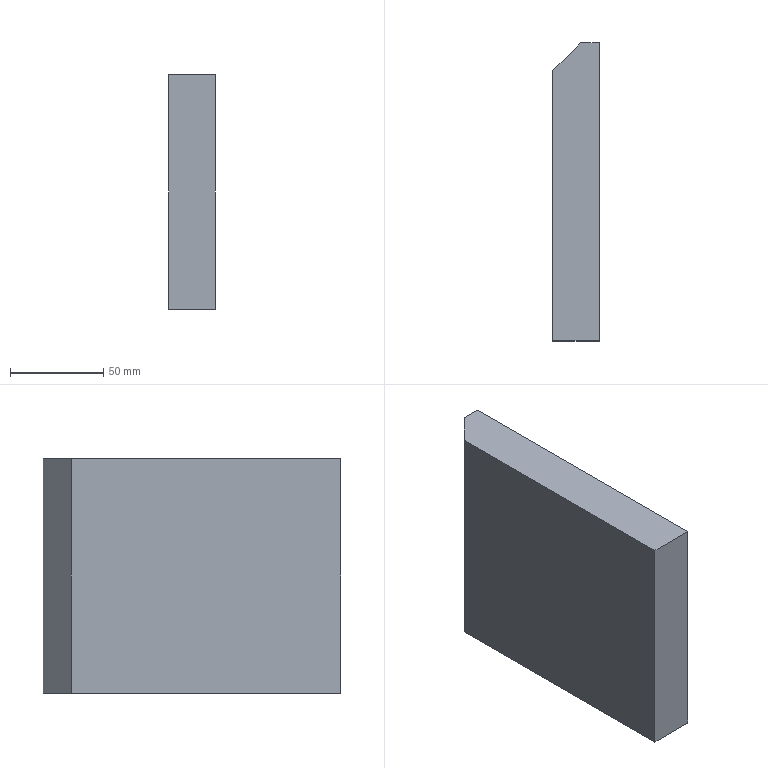Part | SolidWorks | features Chamfer 1, Extrusion 1 | 1 solid | 7 faces | box 25 x 160 x 126 mm | volume 489825 mm3 | plane 7
STEP:
#1=CARTESIAN_POINT('',(-12.5,65.,63.));
#2=VERTEX_POINT('',#1);
#3=CARTESIAN_POINT('',(-12.5,-80.,63.));
#4=VERTEX_POINT('',#3);
#5=CARTESIAN_POINT('',(-12.5,80.,63.));
#6=DIRECTION('',(0.,-1.,0.));
#7=VECTOR('',#6,1000.);
#8=LINE('',#5,#7);
#9=EDGE_CURVE('',#2,#4,#8,.T.);
#10=ORIENTED_EDGE('',*,*,#9,.F.);
#11=CARTESIAN_POINT('',(-12.5,65.,-63.));
#12=VERTEX_POINT('',#11);
#13=CARTESIAN_POINT('',(-12.5,65.,-63.));
#14=DIRECTION('',(0.,0.,-1.));
#15=VECTOR('',#14,1000.);
#16=LINE('',#13,#15);
#17=EDGE_CURVE('',#2,#12,#16,.T.);
#18=ORIENTED_EDGE('',*,*,#17,.T.);
#19=CARTESIAN_POINT('',(-12.5,-80.,-63.));
#20=VERTEX_POINT('',#19);
#21=CARTESIAN_POINT('',(-12.5,80.,-63.));
#22=DIRECTION('',(0.,-1.,0.));
#23=VECTOR('',#22,1000.);
#24=LINE('',#21,#23);
#25=EDGE_CURVE('',#12,#20,#24,.T.);
#26=ORIENTED_EDGE('',*,*,#25,.T.);
#27=CARTESIAN_POINT('',(-12.5,-80.,-63.));
#28=DIRECTION('',(0.,0.,1.));
#29=VECTOR('',#28,1000.);
#30=LINE('',#27,#29);
#31=EDGE_CURVE('',#20,#4,#30,.T.);
#32=ORIENTED_EDGE('',*,*,#31,.T.);
#33=EDGE_LOOP('',(#10,#18,#26,#32));
#34=FACE_OUTER_BOUND('',#33,.T.);
#35=CARTESIAN_POINT('',(-12.5,80.,-63.));
#36=DIRECTION('',(1.,0.,0.));
#37=DIRECTION('',(0.,0.,-1.));
#38=AXIS2_PLACEMENT_3D('',#35,#36,#37);
#39=PLANE('',#38);
#40=ADVANCED_FACE('',(#34),#39,.F.);
#41=CARTESIAN_POINT('',(2.5,80.,63.));
#42=VERTEX_POINT('',#41);
#43=CARTESIAN_POINT('',(12.5,80.,63.));
#44=VERTEX_POINT('',#43);
#45=CARTESIAN_POINT('',(-12.5,80.,63.));
#46=DIRECTION('',(1.,0.,0.));
#47=VECTOR('',#46,1000.);
#48=LINE('',#45,#47);
#49=EDGE_CURVE('',#42,#44,#48,.T.);
#50=ORIENTED_EDGE('',*,*,#49,.F.);
#51=CARTESIAN_POINT('',(2.5,80.,63.));
#52=DIRECTION('',(-0.7071,-0.7071,0.));
#53=VECTOR('',#52,1000.);
#54=LINE('',#51,#53);
#55=EDGE_CURVE('',#42,#2,#54,.T.);
#56=ORIENTED_EDGE('',*,*,#55,.T.);
#57=ORIENTED_EDGE('',*,*,#9,.T.);
#58=CARTESIAN_POINT('',(12.5,-80.,63.));
#59=VERTEX_POINT('',#58);
#60=CARTESIAN_POINT('',(-12.5,-80.,63.));
#61=DIRECTION('',(1.,0.,0.));
#62=VECTOR('',#61,1000.);
#63=LINE('',#60,#62);
#64=EDGE_CURVE('',#4,#59,#63,.T.);
#65=ORIENTED_EDGE('',*,*,#64,.T.);
#66=CARTESIAN_POINT('',(12.5,80.,63.));
#67=DIRECTION('',(0.,-1.,0.));
#68=VECTOR('',#67,1000.);
#69=LINE('',#66,#68);
#70=EDGE_CURVE('',#44,#59,#69,.T.);
#71=ORIENTED_EDGE('',*,*,#70,.F.);
#72=EDGE_LOOP('',(#50,#56,#57,#65,#71));
#73=FACE_OUTER_BOUND('',#72,.T.);
#74=CARTESIAN_POINT('',(-12.5,80.,63.));
#75=DIRECTION('',(0.,0.,-1.));
#76=DIRECTION('',(-1.,0.,0.));
#77=AXIS2_PLACEMENT_3D('',#74,#75,#76);
#78=PLANE('',#77);
#79=ADVANCED_FACE('',(#73),#78,.F.);
#80=CARTESIAN_POINT('',(12.5,-80.,-63.));
#81=VERTEX_POINT('',#80);
#82=CARTESIAN_POINT('',(12.5,-80.,-63.));
#83=DIRECTION('',(0.,0.,-1.));
#84=VECTOR('',#83,1000.);
#85=LINE('',#82,#84);
#86=EDGE_CURVE('',#59,#81,#85,.T.);
#87=ORIENTED_EDGE('',*,*,#86,.T.);
#88=CARTESIAN_POINT('',(12.5,80.,-63.));
#89=VERTEX_POINT('',#88);
#90=CARTESIAN_POINT('',(12.5,80.,-63.));
#91=DIRECTION('',(0.,-1.,0.));
#92=VECTOR('',#91,1000.);
#93=LINE('',#90,#92);
#94=EDGE_CURVE('',#89,#81,#93,.T.);
#95=ORIENTED_EDGE('',*,*,#94,.F.);
#96=CARTESIAN_POINT('',(12.5,80.,-63.));
#97=DIRECTION('',(0.,0.,-1.));
#98=VECTOR('',#97,1000.);
#99=LINE('',#96,#98);
#100=EDGE_CURVE('',#44,#89,#99,.T.);
#101=ORIENTED_EDGE('',*,*,#100,.F.);
#102=ORIENTED_EDGE('',*,*,#70,.T.);
#103=EDGE_LOOP('',(#87,#95,#101,#102));
#104=FACE_OUTER_BOUND('',#103,.T.);
#105=CARTESIAN_POINT('',(12.5,80.,-63.));
#106=DIRECTION('',(-1.,0.,0.));
#107=DIRECTION('',(0.,0.,1.));
#108=AXIS2_PLACEMENT_3D('',#105,#106,#107);
#109=PLANE('',#108);
#110=ADVANCED_FACE('',(#104),#109,.F.);
#111=ORIENTED_EDGE('',*,*,#25,.F.);
#112=CARTESIAN_POINT('',(2.5,80.,-63.));
#113=VERTEX_POINT('',#112);
#114=CARTESIAN_POINT('',(2.5,80.,-63.));
#115=DIRECTION('',(0.7071,0.7071,0.));
#116=VECTOR('',#115,1000.);
#117=LINE('',#114,#116);
#118=EDGE_CURVE('',#12,#113,#117,.T.);
#119=ORIENTED_EDGE('',*,*,#118,.T.);
#120=CARTESIAN_POINT('',(-12.5,80.,-63.));
#121=DIRECTION('',(-1.,0.,0.));
#122=VECTOR('',#121,1000.);
#123=LINE('',#120,#122);
#124=EDGE_CURVE('',#89,#113,#123,.T.);
#125=ORIENTED_EDGE('',*,*,#124,.F.);
#126=ORIENTED_EDGE('',*,*,#94,.T.);
#127=CARTESIAN_POINT('',(-12.5,-80.,-63.));
#128=DIRECTION('',(-1.,0.,0.));
#129=VECTOR('',#128,1000.);
#130=LINE('',#127,#129);
#131=EDGE_CURVE('',#81,#20,#130,.T.);
#132=ORIENTED_EDGE('',*,*,#131,.T.);
#133=EDGE_LOOP('',(#111,#119,#125,#126,#132));
#134=FACE_OUTER_BOUND('',#133,.T.);
#135=CARTESIAN_POINT('',(-12.5,80.,-63.));
#136=DIRECTION('',(0.,0.,1.));
#137=DIRECTION('',(1.,0.,0.));
#138=AXIS2_PLACEMENT_3D('',#135,#136,#137);
#139=PLANE('',#138);
#140=ADVANCED_FACE('',(#134),#139,.F.);
#141=ORIENTED_EDGE('',*,*,#124,.T.);
#142=CARTESIAN_POINT('',(2.5,80.,63.));
#143=DIRECTION('',(0.,0.,1.));
#144=VECTOR('',#143,1000.);
#145=LINE('',#142,#144);
#146=EDGE_CURVE('',#113,#42,#145,.T.);
#147=ORIENTED_EDGE('',*,*,#146,.T.);
#148=ORIENTED_EDGE('',*,*,#49,.T.);
#149=ORIENTED_EDGE('',*,*,#100,.T.);
#150=EDGE_LOOP('',(#141,#147,#148,#149));
#151=FACE_OUTER_BOUND('',#150,.T.);
#152=CARTESIAN_POINT('',(0.,80.,0.));
#153=DIRECTION('',(0.,1.,0.));
#154=DIRECTION('',(0.,0.,1.));
#155=AXIS2_PLACEMENT_3D('',#152,#153,#154);
#156=PLANE('',#155);
#157=ADVANCED_FACE('',(#151),#156,.T.);
#158=ORIENTED_EDGE('',*,*,#31,.F.);
#159=ORIENTED_EDGE('',*,*,#131,.F.);
#160=ORIENTED_EDGE('',*,*,#86,.F.);
#161=ORIENTED_EDGE('',*,*,#64,.F.);
#162=EDGE_LOOP('',(#158,#159,#160,#161));
#163=FACE_OUTER_BOUND('',#162,.T.);
#164=CARTESIAN_POINT('',(0.,-80.,0.));
#165=DIRECTION('',(0.,1.,0.));
#166=DIRECTION('',(0.,0.,1.));
#167=AXIS2_PLACEMENT_3D('',#164,#165,#166);
#168=PLANE('',#167);
#169=ADVANCED_FACE('',(#163),#168,.F.);
#170=ORIENTED_EDGE('',*,*,#118,.F.);
#171=ORIENTED_EDGE('',*,*,#17,.F.);
#172=ORIENTED_EDGE('',*,*,#55,.F.);
#173=ORIENTED_EDGE('',*,*,#146,.F.);
#174=EDGE_LOOP('',(#170,#171,#172,#173));
#175=FACE_OUTER_BOUND('',#174,.T.);
#176=CARTESIAN_POINT('',(2.5,80.,0.));
#177=DIRECTION('',(-0.7071,0.7071,0.));
#178=DIRECTION('',(0.,0.,-1.));
#179=AXIS2_PLACEMENT_3D('',#176,#177,#178);
#180=PLANE('',#179);
#181=ADVANCED_FACE('',(#175),#180,.T.);
#182=CLOSED_SHELL('',(#40,#79,#110,#140,#157,#169,#181));
#183=MANIFOLD_SOLID_BREP('',#182);
#184=CARTESIAN_POINT('',(0.,0.,0.));
#185=DIRECTION('',(0.,0.,1.));
#186=DIRECTION('',(1.,0.,0.));
#187=AXIS2_PLACEMENT_3D('',#184,#185,#186);
#188=(LENGTH_UNIT()NAMED_UNIT(*)SI_UNIT(.MILLI.,.METRE.));
#189=UNCERTAINTY_MEASURE_WITH_UNIT(LENGTH_MEASURE(0.00001),#188,'','');
#190=(NAMED_UNIT(*)PLANE_ANGLE_UNIT()SI_UNIT($,.RADIAN.));
#191=(NAMED_UNIT(*)SI_UNIT($,.STERADIAN.)SOLID_ANGLE_UNIT());
#192=(GEOMETRIC_REPRESENTATION_CONTEXT(3)GLOBAL_UNCERTAINTY_ASSIGNED_CONTEXT((#189))GLOBAL_UNIT_ASSIGNED_CONTEXT((#188,#190,#191))REPRESENTATION_CONTEXT('',''));
#193=ADVANCED_BREP_SHAPE_REPRESENTATION('',(#183,#187),#192);